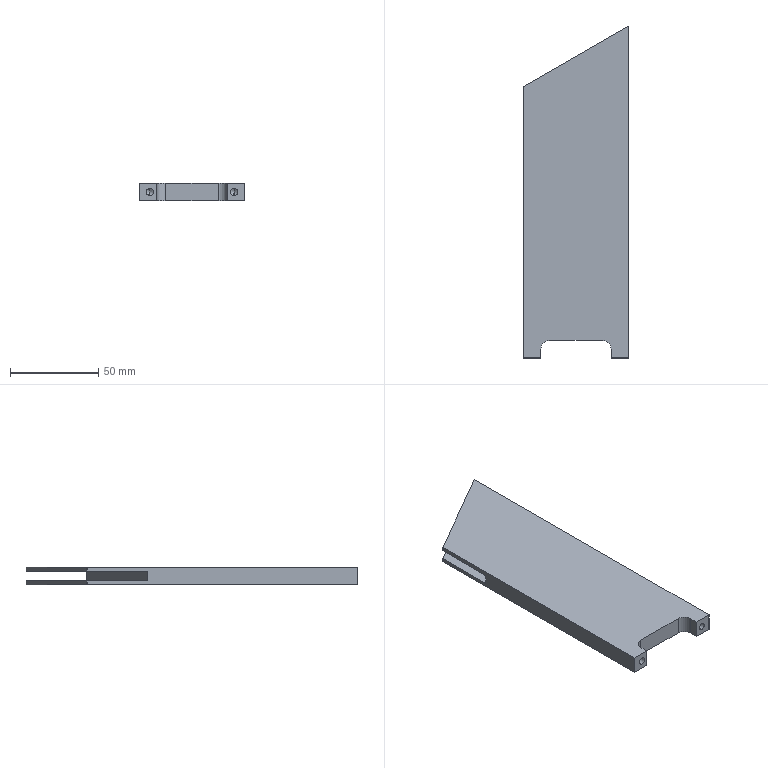Part | STEP file | GLSJ-10-32_default | 1 solid | 32 faces | box 60 x 188.591 x 10 mm | volume 87112 mm3 | plane 22 | cylinder 6 | cone 4 | commonest cylinder face diameters 4.2 x4 10 x2